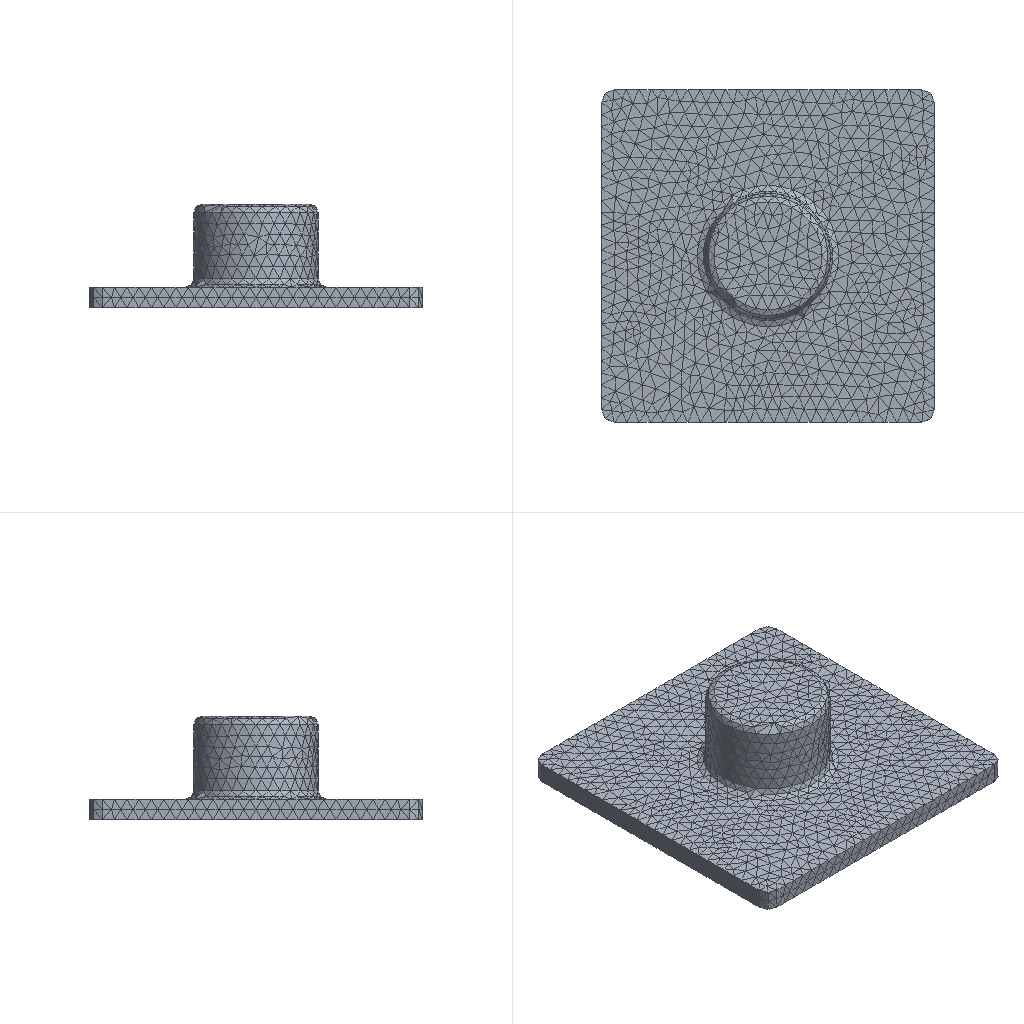Simulation study | ansys workbench
Set-up summary:
category,name,step,type,value,unit,region
solver,ansys_workbench
units,mm-N-s-tonne (MPa),,stated,"/units,MPA"
analysis,deck-1/LS1,,steady-state thermal
load_step,deck-1/LS1,deck-1/LS1,steady-state thermal,nsubst=1; time=1
analysis,deck-2/LS1,,static
load_step,deck-2/LS1,deck-2/LS1,static,nsubst=1; time=1
mesh,deck-1.dat,,nodes,24489
mesh,deck-1.dat,,elements,19249
element_type,SOLID291,,,15247,,deck-1.dat
element_type,SURF152,,,4002,,deck-1.dat
mesh,deck-2.dat,,nodes,24489
mesh,deck-2.dat,,elements,15247
element_type,SOLID187,,,15247,,deck-2.dat
material,Structural Steel,,E,200000,tonne s^-2 mm^-1
material,Structural Steel,,nu,0.3
material,Structural Steel,,density,7.85e-09,tonne mm^-3
material,Structural Steel,,conductivity,60.5,tonne mm s^-3 C^-1
material,Structural Steel,,specific_heat,4.34e+08,mm^2 s^-2 C^-1
material,Structural Steel,,cte,1.2e-05,C^-1
material,Structural Steel,,permeability,10000
material,Structural Steel,,resistivity,0.00017,ohm mm
load,Define Uniform Initial temperature,deck-1/model,body load temp,22,,all
load,"Create ""______""",deck-1/LS1,convection,0.0124,,SURF152 #2
bc,,deck-1/LS1,temperature,150 [dofs=TEMP n=3],,node list
bc,Fixed Supports,deck-2/model,fixed,[dofs=ALL],,_FIXEDSU
named_set,_CM32,,node,281
named_set,_CM34,,node,3125
named_set,_CM45,,node,840
named_set,_FIXEDSU,,node,3125
gap,"BFBLOCK present, not parsed (24489 lines)"
Results summary:
result,analyses[0].index,,,1
result,analyses[0].system,,,SYS
result,analyses[0].deck,,,deck-1.dat
result,analyses[0].solve_status,,,completed
result,analyses[0].analysis_type,,,static
result,analyses[0].physics,,,thermal
result,analyses[0].unit_system,,,"NMM: mm, ton, N, s, mV, mA, degC"
result,analyses[0].n_sets,,,1
result,analyses[0].load_steps[0].set,set=1,,1
result,analyses[0].load_steps[0].time_or_freq,set=1,,1
result,analyses[0].load_steps[0].max_temperature,set=1,,150
result,analyses[0].load_steps[0].min_temperature,set=1,,29.998
result,analyses[1].index,,,2
result,analyses[1].system,,,SYS-1
result,analyses[1].deck,,,deck-2.dat
result,analyses[1].solve_status,,,completed
result,analyses[1].analysis_type,,,static
result,analyses[1].physics,,,mechanical
result,analyses[1].unit_system,,,"NMM: mm, ton, N, s, mV, mA, degC"
result,analyses[1].n_sets,,,1
result,analyses[1].load_steps[0].set,set=1,,1
result,analyses[1].load_steps[0].time_or_freq,set=1,,1
result,analyses[1].load_steps[0].max_displacement_magnitude,set=1,,0.02547
result,analyses[1].load_steps[0].max_von_mises_nodal,set=1,,206.489
result,analyses[1].load_steps[0].reaction_force_sum_xyz[1],set=1,,6.57015e-06
result,analyses[1].load_steps[0].reaction_force_sum_xyz[2],set=1,,5.09897e-05
result,analyses[1].load_steps[0].reaction_force_sum_xyz[3],set=1,,-6.78665e-05